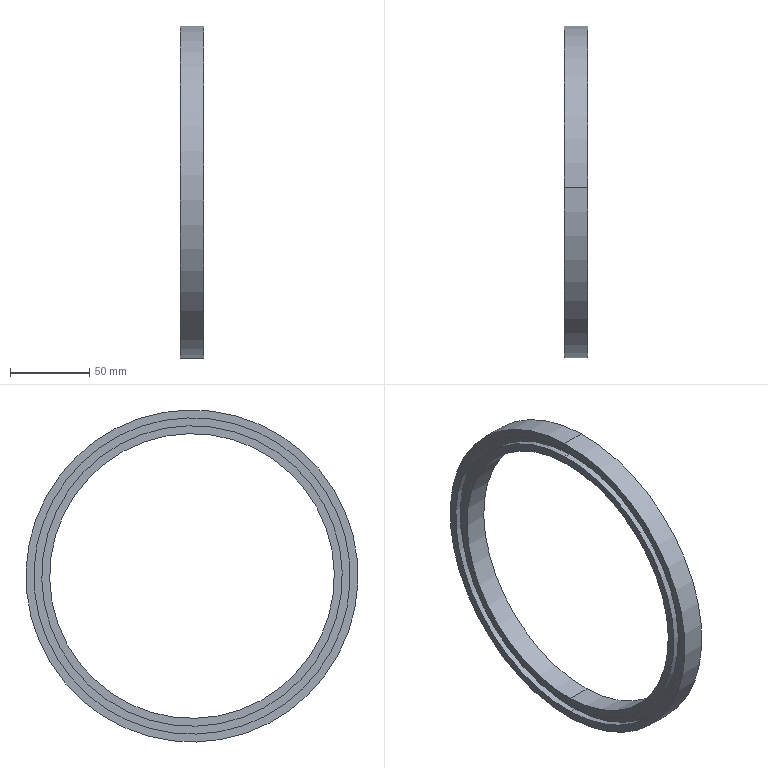Part | NX | features BREP 1 | 1 solid | 18 faces | box 15 x 210 x 210 mm | volume 113333 mm3 | cylinder 12 | plane 6 | commonest cylinder face diameters 190 x4 200 x4 180 x2 210 x2
STEP:
#1=CARTESIAN_POINT('',(-426.355,2.532,94.966));
#2=VERTEX_POINT('',#1);
#3=CARTESIAN_POINT('',(-426.355,-2.532,-94.966));
#4=VERTEX_POINT('',#3);
#5=CARTESIAN_POINT('',(-426.355,0.,0.));
#6=DIRECTION('',(1.,0.,0.));
#7=DIRECTION('',(0.,0.02665,0.9996));
#8=AXIS2_PLACEMENT_3D('',#5,#6,#7);
#9=CIRCLE('',#8,95.);
#10=EDGE_CURVE('',#2,#4,#9,.T.);
#11=ORIENTED_EDGE('',*,*,#10,.T.);
#12=CARTESIAN_POINT('',(-422.355,-2.532,-94.966));
#13=VERTEX_POINT('',#12);
#14=CARTESIAN_POINT('',(-429.855,-2.532,-94.966));
#15=DIRECTION('',(-1.,0.,0.));
#16=VECTOR('',#15,1000.);
#17=LINE('',#14,#16);
#18=EDGE_CURVE('',#4,#13,#17,.F.);
#19=ORIENTED_EDGE('',*,*,#18,.T.);
#20=CARTESIAN_POINT('',(-422.355,2.532,94.966));
#21=VERTEX_POINT('',#20);
#22=CARTESIAN_POINT('',(-422.355,0.,0.));
#23=DIRECTION('',(1.,0.,0.));
#24=DIRECTION('',(0.,0.02665,0.9996));
#25=AXIS2_PLACEMENT_3D('',#22,#23,#24);
#26=CIRCLE('',#25,95.);
#27=EDGE_CURVE('',#21,#13,#26,.T.);
#28=ORIENTED_EDGE('',*,*,#27,.F.);
#29=CARTESIAN_POINT('',(-429.855,2.532,94.966));
#30=DIRECTION('',(-1.,0.,0.));
#31=VECTOR('',#30,1000.);
#32=LINE('',#29,#31);
#33=EDGE_CURVE('',#2,#21,#32,.F.);
#34=ORIENTED_EDGE('',*,*,#33,.F.);
#35=EDGE_LOOP('',(#11,#19,#28,#34));
#36=FACE_BOUND('',#35,.T.);
#37=CARTESIAN_POINT('',(-429.855,0.,0.));
#38=DIRECTION('',(1.,0.,0.));
#39=DIRECTION('',(0.,0.02665,0.9996));
#40=AXIS2_PLACEMENT_3D('',#37,#38,#39);
#41=CYLINDRICAL_SURFACE('',#40,95.);
#42=ADVANCED_FACE('',(#36),#41,.T.);
#43=CARTESIAN_POINT('',(-426.355,-2.665,-99.964));
#44=VERTEX_POINT('',#43);
#45=CARTESIAN_POINT('',(-426.355,2.665,99.964));
#46=VERTEX_POINT('',#45);
#47=CARTESIAN_POINT('',(-426.355,0.,0.));
#48=DIRECTION('',(1.,0.,0.));
#49=DIRECTION('',(0.,0.02665,0.9996));
#50=AXIS2_PLACEMENT_3D('',#47,#48,#49);
#51=CIRCLE('',#50,100.);
#52=EDGE_CURVE('',#44,#46,#51,.T.);
#53=ORIENTED_EDGE('',*,*,#52,.F.);
#54=CARTESIAN_POINT('',(-422.355,-2.665,-99.964));
#55=VERTEX_POINT('',#54);
#56=CARTESIAN_POINT('',(-429.855,-2.665,-99.964));
#57=DIRECTION('',(-1.,0.,0.));
#58=VECTOR('',#57,1000.);
#59=LINE('',#56,#58);
#60=EDGE_CURVE('',#44,#55,#59,.F.);
#61=ORIENTED_EDGE('',*,*,#60,.T.);
#62=CARTESIAN_POINT('',(-422.355,2.665,99.964));
#63=VERTEX_POINT('',#62);
#64=CARTESIAN_POINT('',(-422.355,0.,0.));
#65=DIRECTION('',(1.,0.,0.));
#66=DIRECTION('',(0.,0.02665,0.9996));
#67=AXIS2_PLACEMENT_3D('',#64,#65,#66);
#68=CIRCLE('',#67,100.);
#69=EDGE_CURVE('',#55,#63,#68,.T.);
#70=ORIENTED_EDGE('',*,*,#69,.T.);
#71=CARTESIAN_POINT('',(-429.855,2.665,99.964));
#72=DIRECTION('',(-1.,0.,0.));
#73=VECTOR('',#72,1000.);
#74=LINE('',#71,#73);
#75=EDGE_CURVE('',#46,#63,#74,.F.);
#76=ORIENTED_EDGE('',*,*,#75,.F.);
#77=EDGE_LOOP('',(#53,#61,#70,#76));
#78=FACE_BOUND('',#77,.T.);
#79=CARTESIAN_POINT('',(-429.855,0.,0.));
#80=DIRECTION('',(1.,0.,0.));
#81=DIRECTION('',(0.,0.02665,0.9996));
#82=AXIS2_PLACEMENT_3D('',#79,#80,#81);
#83=CYLINDRICAL_SURFACE('',#82,100.);
#84=ADVANCED_FACE('',(#78),#83,.F.);
#85=CARTESIAN_POINT('',(-437.355,2.798,104.963));
#86=VERTEX_POINT('',#85);
#87=CARTESIAN_POINT('',(-437.355,-2.798,-104.963));
#88=VERTEX_POINT('',#87);
#89=CARTESIAN_POINT('',(-437.355,0.,0.));
#90=DIRECTION('',(1.,0.,0.));
#91=DIRECTION('',(0.,0.02665,0.9996));
#92=AXIS2_PLACEMENT_3D('',#89,#90,#91);
#93=CIRCLE('',#92,105.);
#94=EDGE_CURVE('',#86,#88,#93,.T.);
#95=ORIENTED_EDGE('',*,*,#94,.T.);
#96=CARTESIAN_POINT('',(-422.355,-2.798,-104.963));
#97=VERTEX_POINT('',#96);
#98=CARTESIAN_POINT('',(-429.855,-2.798,-104.963));
#99=DIRECTION('',(-1.,0.,0.));
#100=VECTOR('',#99,1000.);
#101=LINE('',#98,#100);
#102=EDGE_CURVE('',#88,#97,#101,.F.);
#103=ORIENTED_EDGE('',*,*,#102,.T.);
#104=CARTESIAN_POINT('',(-422.355,2.798,104.963));
#105=VERTEX_POINT('',#104);
#106=CARTESIAN_POINT('',(-422.355,0.,0.));
#107=DIRECTION('',(1.,0.,0.));
#108=DIRECTION('',(0.,0.02665,0.9996));
#109=AXIS2_PLACEMENT_3D('',#106,#107,#108);
#110=CIRCLE('',#109,105.);
#111=EDGE_CURVE('',#105,#97,#110,.T.);
#112=ORIENTED_EDGE('',*,*,#111,.F.);
#113=CARTESIAN_POINT('',(-429.855,2.798,104.963));
#114=DIRECTION('',(-1.,0.,0.));
#115=VECTOR('',#114,1000.);
#116=LINE('',#113,#115);
#117=EDGE_CURVE('',#86,#105,#116,.F.);
#118=ORIENTED_EDGE('',*,*,#117,.F.);
#119=EDGE_LOOP('',(#95,#103,#112,#118));
#120=FACE_BOUND('',#119,.T.);
#121=CARTESIAN_POINT('',(-429.855,0.,0.));
#122=DIRECTION('',(1.,0.,0.));
#123=DIRECTION('',(0.,0.02665,0.9996));
#124=AXIS2_PLACEMENT_3D('',#121,#122,#123);
#125=CYLINDRICAL_SURFACE('',#124,105.);
#126=ADVANCED_FACE('',(#120),#125,.T.);
#127=CARTESIAN_POINT('',(-437.355,-2.665,-99.964));
#128=VERTEX_POINT('',#127);
#129=CARTESIAN_POINT('',(-437.355,2.665,99.964));
#130=VERTEX_POINT('',#129);
#131=CARTESIAN_POINT('',(-437.355,0.,0.));
#132=DIRECTION('',(1.,0.,0.));
#133=DIRECTION('',(0.,0.02665,0.9996));
#134=AXIS2_PLACEMENT_3D('',#131,#132,#133);
#135=CIRCLE('',#134,100.);
#136=EDGE_CURVE('',#128,#130,#135,.T.);
#137=ORIENTED_EDGE('',*,*,#136,.F.);
#138=CARTESIAN_POINT('',(-433.355,-2.665,-99.964));
#139=VERTEX_POINT('',#138);
#140=CARTESIAN_POINT('',(-429.855,-2.665,-99.964));
#141=DIRECTION('',(-1.,0.,0.));
#142=VECTOR('',#141,1000.);
#143=LINE('',#140,#142);
#144=EDGE_CURVE('',#128,#139,#143,.F.);
#145=ORIENTED_EDGE('',*,*,#144,.T.);
#146=CARTESIAN_POINT('',(-433.355,2.665,99.964));
#147=VERTEX_POINT('',#146);
#148=CARTESIAN_POINT('',(-433.355,0.,0.));
#149=DIRECTION('',(1.,0.,0.));
#150=DIRECTION('',(0.,0.02665,0.9996));
#151=AXIS2_PLACEMENT_3D('',#148,#149,#150);
#152=CIRCLE('',#151,100.);
#153=EDGE_CURVE('',#139,#147,#152,.T.);
#154=ORIENTED_EDGE('',*,*,#153,.T.);
#155=CARTESIAN_POINT('',(-429.855,2.665,99.964));
#156=DIRECTION('',(-1.,0.,0.));
#157=VECTOR('',#156,1000.);
#158=LINE('',#155,#157);
#159=EDGE_CURVE('',#130,#147,#158,.F.);
#160=ORIENTED_EDGE('',*,*,#159,.F.);
#161=EDGE_LOOP('',(#137,#145,#154,#160));
#162=FACE_BOUND('',#161,.T.);
#163=CARTESIAN_POINT('',(-429.855,0.,0.));
#164=DIRECTION('',(1.,0.,0.));
#165=DIRECTION('',(0.,0.02665,0.9996));
#166=AXIS2_PLACEMENT_3D('',#163,#164,#165);
#167=CYLINDRICAL_SURFACE('',#166,100.);
#168=ADVANCED_FACE('',(#162),#167,.F.);
#169=CARTESIAN_POINT('',(-437.355,2.532,94.966));
#170=VERTEX_POINT('',#169);
#171=CARTESIAN_POINT('',(-437.355,-2.532,-94.966));
#172=VERTEX_POINT('',#171);
#173=CARTESIAN_POINT('',(-437.355,0.,0.));
#174=DIRECTION('',(1.,0.,0.));
#175=DIRECTION('',(0.,0.02665,0.9996));
#176=AXIS2_PLACEMENT_3D('',#173,#174,#175);
#177=CIRCLE('',#176,95.);
#178=EDGE_CURVE('',#170,#172,#177,.T.);
#179=ORIENTED_EDGE('',*,*,#178,.T.);
#180=CARTESIAN_POINT('',(-433.355,-2.532,-94.966));
#181=VERTEX_POINT('',#180);
#182=CARTESIAN_POINT('',(-429.855,-2.532,-94.966));
#183=DIRECTION('',(-1.,0.,0.));
#184=VECTOR('',#183,1000.);
#185=LINE('',#182,#184);
#186=EDGE_CURVE('',#172,#181,#185,.F.);
#187=ORIENTED_EDGE('',*,*,#186,.T.);
#188=CARTESIAN_POINT('',(-433.355,2.532,94.966));
#189=VERTEX_POINT('',#188);
#190=CARTESIAN_POINT('',(-433.355,0.,0.));
#191=DIRECTION('',(1.,0.,0.));
#192=DIRECTION('',(0.,0.02665,0.9996));
#193=AXIS2_PLACEMENT_3D('',#190,#191,#192);
#194=CIRCLE('',#193,95.);
#195=EDGE_CURVE('',#189,#181,#194,.T.);
#196=ORIENTED_EDGE('',*,*,#195,.F.);
#197=CARTESIAN_POINT('',(-429.855,2.532,94.966));
#198=DIRECTION('',(-1.,0.,0.));
#199=VECTOR('',#198,1000.);
#200=LINE('',#197,#199);
#201=EDGE_CURVE('',#170,#189,#200,.F.);
#202=ORIENTED_EDGE('',*,*,#201,.F.);
#203=EDGE_LOOP('',(#179,#187,#196,#202));
#204=FACE_BOUND('',#203,.T.);
#205=CARTESIAN_POINT('',(-429.855,0.,0.));
#206=DIRECTION('',(1.,0.,0.));
#207=DIRECTION('',(0.,0.02665,0.9996));
#208=AXIS2_PLACEMENT_3D('',#205,#206,#207);
#209=CYLINDRICAL_SURFACE('',#208,95.);
#210=ADVANCED_FACE('',(#204),#209,.T.);
#211=CARTESIAN_POINT('',(-437.355,-2.399,-89.968));
#212=VERTEX_POINT('',#211);
#213=CARTESIAN_POINT('',(-437.355,2.399,89.968));
#214=VERTEX_POINT('',#213);
#215=CARTESIAN_POINT('',(-437.355,0.,0.));
#216=DIRECTION('',(1.,0.,0.));
#217=DIRECTION('',(0.,0.02665,0.9996));
#218=AXIS2_PLACEMENT_3D('',#215,#216,#217);
#219=CIRCLE('',#218,90.);
#220=EDGE_CURVE('',#212,#214,#219,.T.);
#221=ORIENTED_EDGE('',*,*,#220,.F.);
#222=CARTESIAN_POINT('',(-422.355,-2.399,-89.968));
#223=VERTEX_POINT('',#222);
#224=CARTESIAN_POINT('',(-429.855,-2.399,-89.968));
#225=DIRECTION('',(-1.,0.,0.));
#226=VECTOR('',#225,1000.);
#227=LINE('',#224,#226);
#228=EDGE_CURVE('',#212,#223,#227,.F.);
#229=ORIENTED_EDGE('',*,*,#228,.T.);
#230=CARTESIAN_POINT('',(-422.355,2.399,89.968));
#231=VERTEX_POINT('',#230);
#232=CARTESIAN_POINT('',(-422.355,0.,0.));
#233=DIRECTION('',(1.,0.,0.));
#234=DIRECTION('',(0.,0.02665,0.9996));
#235=AXIS2_PLACEMENT_3D('',#232,#233,#234);
#236=CIRCLE('',#235,90.);
#237=EDGE_CURVE('',#223,#231,#236,.T.);
#238=ORIENTED_EDGE('',*,*,#237,.T.);
#239=CARTESIAN_POINT('',(-429.855,2.399,89.968));
#240=DIRECTION('',(-1.,0.,0.));
#241=VECTOR('',#240,1000.);
#242=LINE('',#239,#241);
#243=EDGE_CURVE('',#214,#231,#242,.F.);
#244=ORIENTED_EDGE('',*,*,#243,.F.);
#245=EDGE_LOOP('',(#221,#229,#238,#244));
#246=FACE_BOUND('',#245,.T.);
#247=CARTESIAN_POINT('',(-429.855,0.,0.));
#248=DIRECTION('',(1.,0.,0.));
#249=DIRECTION('',(0.,0.02665,0.9996));
#250=AXIS2_PLACEMENT_3D('',#247,#248,#249);
#251=CYLINDRICAL_SURFACE('',#250,90.);
#252=ADVANCED_FACE('',(#246),#251,.F.);
#253=ORIENTED_EDGE('',*,*,#228,.F.);
#254=CARTESIAN_POINT('',(-437.355,0.,0.));
#255=DIRECTION('',(1.,0.,0.));
#256=DIRECTION('',(0.,0.02665,0.9996));
#257=AXIS2_PLACEMENT_3D('',#254,#255,#256);
#258=CIRCLE('',#257,90.);
#259=EDGE_CURVE('',#214,#212,#258,.T.);
#260=ORIENTED_EDGE('',*,*,#259,.F.);
#261=ORIENTED_EDGE('',*,*,#243,.T.);
#262=CARTESIAN_POINT('',(-422.355,0.,0.));
#263=DIRECTION('',(1.,0.,0.));
#264=DIRECTION('',(0.,0.02665,0.9996));
#265=AXIS2_PLACEMENT_3D('',#262,#263,#264);
#266=CIRCLE('',#265,90.);
#267=EDGE_CURVE('',#231,#223,#266,.T.);
#268=ORIENTED_EDGE('',*,*,#267,.T.);
#269=EDGE_LOOP('',(#253,#260,#261,#268));
#270=FACE_BOUND('',#269,.T.);
#271=CARTESIAN_POINT('',(-429.855,0.,0.));
#272=DIRECTION('',(1.,0.,0.));
#273=DIRECTION('',(0.,0.02665,0.9996));
#274=AXIS2_PLACEMENT_3D('',#271,#272,#273);
#275=CYLINDRICAL_SURFACE('',#274,90.);
#276=ADVANCED_FACE('',(#270),#275,.F.);
#277=ORIENTED_EDGE('',*,*,#178,.F.);
#278=CARTESIAN_POINT('',(-437.355,0.,0.));
#279=DIRECTION('',(1.,0.,0.));
#280=DIRECTION('',(0.,0.02665,0.9996));
#281=AXIS2_PLACEMENT_3D('',#278,#279,#280);
#282=CIRCLE('',#281,95.);
#283=EDGE_CURVE('',#172,#170,#282,.T.);
#284=ORIENTED_EDGE('',*,*,#283,.F.);
#285=EDGE_LOOP('',(#277,#284));
#286=FACE_BOUND('',#285,.T.);
#287=ORIENTED_EDGE('',*,*,#259,.T.);
#288=ORIENTED_EDGE('',*,*,#220,.T.);
#289=EDGE_LOOP('',(#287,#288));
#290=FACE_BOUND('',#289,.T.);
#291=CARTESIAN_POINT('',(-437.355,-89.968,2.399));
#292=DIRECTION('',(1.,0.,0.));
#293=DIRECTION('',(0.,0.02665,0.9996));
#294=AXIS2_PLACEMENT_3D('',#291,#292,#293);
#295=PLANE('',#294);
#296=ADVANCED_FACE('',(#286,#290),#295,.F.);
#297=ORIENTED_EDGE('',*,*,#186,.F.);
#298=ORIENTED_EDGE('',*,*,#283,.T.);
#299=ORIENTED_EDGE('',*,*,#201,.T.);
#300=CARTESIAN_POINT('',(-433.355,0.,0.));
#301=DIRECTION('',(1.,0.,0.));
#302=DIRECTION('',(0.,0.02665,0.9996));
#303=AXIS2_PLACEMENT_3D('',#300,#301,#302);
#304=CIRCLE('',#303,95.);
#305=EDGE_CURVE('',#181,#189,#304,.T.);
#306=ORIENTED_EDGE('',*,*,#305,.F.);
#307=EDGE_LOOP('',(#297,#298,#299,#306));
#308=FACE_BOUND('',#307,.T.);
#309=CARTESIAN_POINT('',(-429.855,0.,0.));
#310=DIRECTION('',(1.,0.,0.));
#311=DIRECTION('',(0.,0.02665,0.9996));
#312=AXIS2_PLACEMENT_3D('',#309,#310,#311);
#313=CYLINDRICAL_SURFACE('',#312,95.);
#314=ADVANCED_FACE('',(#308),#313,.T.);
#315=CARTESIAN_POINT('',(-433.355,0.,0.));
#316=DIRECTION('',(1.,0.,0.));
#317=DIRECTION('',(0.,0.02665,0.9996));
#318=AXIS2_PLACEMENT_3D('',#315,#316,#317);
#319=CIRCLE('',#318,100.);
#320=EDGE_CURVE('',#147,#139,#319,.T.);
#321=ORIENTED_EDGE('',*,*,#320,.F.);
#322=ORIENTED_EDGE('',*,*,#153,.F.);
#323=EDGE_LOOP('',(#321,#322));
#324=FACE_BOUND('',#323,.T.);
#325=ORIENTED_EDGE('',*,*,#195,.T.);
#326=ORIENTED_EDGE('',*,*,#305,.T.);
#327=EDGE_LOOP('',(#325,#326));
#328=FACE_BOUND('',#327,.T.);
#329=CARTESIAN_POINT('',(-433.355,-94.966,2.532));
#330=DIRECTION('',(1.,0.,0.));
#331=DIRECTION('',(0.,0.02665,0.9996));
#332=AXIS2_PLACEMENT_3D('',#329,#330,#331);
#333=PLANE('',#332);
#334=ADVANCED_FACE('',(#324,#328),#333,.F.);
#335=ORIENTED_EDGE('',*,*,#144,.F.);
#336=CARTESIAN_POINT('',(-437.355,0.,0.));
#337=DIRECTION('',(1.,0.,0.));
#338=DIRECTION('',(0.,0.02665,0.9996));
#339=AXIS2_PLACEMENT_3D('',#336,#337,#338);
#340=CIRCLE('',#339,100.);
#341=EDGE_CURVE('',#130,#128,#340,.T.);
#342=ORIENTED_EDGE('',*,*,#341,.F.);
#343=ORIENTED_EDGE('',*,*,#159,.T.);
#344=ORIENTED_EDGE('',*,*,#320,.T.);
#345=EDGE_LOOP('',(#335,#342,#343,#344));
#346=FACE_BOUND('',#345,.T.);
#347=CARTESIAN_POINT('',(-429.855,0.,0.));
#348=DIRECTION('',(1.,0.,0.));
#349=DIRECTION('',(0.,0.02665,0.9996));
#350=AXIS2_PLACEMENT_3D('',#347,#348,#349);
#351=CYLINDRICAL_SURFACE('',#350,100.);
#352=ADVANCED_FACE('',(#346),#351,.F.);
#353=ORIENTED_EDGE('',*,*,#94,.F.);
#354=CARTESIAN_POINT('',(-437.355,0.,0.));
#355=DIRECTION('',(1.,0.,0.));
#356=DIRECTION('',(0.,0.02665,0.9996));
#357=AXIS2_PLACEMENT_3D('',#354,#355,#356);
#358=CIRCLE('',#357,105.);
#359=EDGE_CURVE('',#88,#86,#358,.T.);
#360=ORIENTED_EDGE('',*,*,#359,.F.);
#361=EDGE_LOOP('',(#353,#360));
#362=FACE_BOUND('',#361,.T.);
#363=ORIENTED_EDGE('',*,*,#341,.T.);
#364=ORIENTED_EDGE('',*,*,#136,.T.);
#365=EDGE_LOOP('',(#363,#364));
#366=FACE_BOUND('',#365,.T.);
#367=CARTESIAN_POINT('',(-437.355,-99.964,2.665));
#368=DIRECTION('',(1.,0.,0.));
#369=DIRECTION('',(0.,0.02665,0.9996));
#370=AXIS2_PLACEMENT_3D('',#367,#368,#369);
#371=PLANE('',#370);
#372=ADVANCED_FACE('',(#362,#366),#371,.F.);
#373=ORIENTED_EDGE('',*,*,#102,.F.);
#374=ORIENTED_EDGE('',*,*,#359,.T.);
#375=ORIENTED_EDGE('',*,*,#117,.T.);
#376=CARTESIAN_POINT('',(-422.355,0.,0.));
#377=DIRECTION('',(1.,0.,0.));
#378=DIRECTION('',(0.,0.02665,0.9996));
#379=AXIS2_PLACEMENT_3D('',#376,#377,#378);
#380=CIRCLE('',#379,105.);
#381=EDGE_CURVE('',#97,#105,#380,.T.);
#382=ORIENTED_EDGE('',*,*,#381,.F.);
#383=EDGE_LOOP('',(#373,#374,#375,#382));
#384=FACE_BOUND('',#383,.T.);
#385=CARTESIAN_POINT('',(-429.855,0.,0.));
#386=DIRECTION('',(1.,0.,0.));
#387=DIRECTION('',(0.,0.02665,0.9996));
#388=AXIS2_PLACEMENT_3D('',#385,#386,#387);
#389=CYLINDRICAL_SURFACE('',#388,105.);
#390=ADVANCED_FACE('',(#384),#389,.T.);
#391=CARTESIAN_POINT('',(-422.355,0.,0.));
#392=DIRECTION('',(1.,0.,0.));
#393=DIRECTION('',(0.,0.02665,0.9996));
#394=AXIS2_PLACEMENT_3D('',#391,#392,#393);
#395=CIRCLE('',#394,100.);
#396=EDGE_CURVE('',#63,#55,#395,.T.);
#397=ORIENTED_EDGE('',*,*,#396,.F.);
#398=ORIENTED_EDGE('',*,*,#69,.F.);
#399=EDGE_LOOP('',(#397,#398));
#400=FACE_BOUND('',#399,.T.);
#401=ORIENTED_EDGE('',*,*,#111,.T.);
#402=ORIENTED_EDGE('',*,*,#381,.T.);
#403=EDGE_LOOP('',(#401,#402));
#404=FACE_BOUND('',#403,.T.);
#405=CARTESIAN_POINT('',(-422.355,-104.963,2.798));
#406=DIRECTION('',(-1.,0.,0.));
#407=DIRECTION('',(0.,-0.02665,-0.9996));
#408=AXIS2_PLACEMENT_3D('',#405,#406,#407);
#409=PLANE('',#408);
#410=ADVANCED_FACE('',(#400,#404),#409,.F.);
#411=ORIENTED_EDGE('',*,*,#60,.F.);
#412=CARTESIAN_POINT('',(-426.355,0.,0.));
#413=DIRECTION('',(1.,0.,0.));
#414=DIRECTION('',(0.,0.02665,0.9996));
#415=AXIS2_PLACEMENT_3D('',#412,#413,#414);
#416=CIRCLE('',#415,100.);
#417=EDGE_CURVE('',#46,#44,#416,.T.);
#418=ORIENTED_EDGE('',*,*,#417,.F.);
#419=ORIENTED_EDGE('',*,*,#75,.T.);
#420=ORIENTED_EDGE('',*,*,#396,.T.);
#421=EDGE_LOOP('',(#411,#418,#419,#420));
#422=FACE_BOUND('',#421,.T.);
#423=CARTESIAN_POINT('',(-429.855,0.,0.));
#424=DIRECTION('',(1.,0.,0.));
#425=DIRECTION('',(0.,0.02665,0.9996));
#426=AXIS2_PLACEMENT_3D('',#423,#424,#425);
#427=CYLINDRICAL_SURFACE('',#426,100.);
#428=ADVANCED_FACE('',(#422),#427,.F.);
#429=ORIENTED_EDGE('',*,*,#10,.F.);
#430=CARTESIAN_POINT('',(-426.355,0.,0.));
#431=DIRECTION('',(1.,0.,0.));
#432=DIRECTION('',(0.,0.02665,0.9996));
#433=AXIS2_PLACEMENT_3D('',#430,#431,#432);
#434=CIRCLE('',#433,95.);
#435=EDGE_CURVE('',#4,#2,#434,.T.);
#436=ORIENTED_EDGE('',*,*,#435,.F.);
#437=EDGE_LOOP('',(#429,#436));
#438=FACE_BOUND('',#437,.T.);
#439=ORIENTED_EDGE('',*,*,#417,.T.);
#440=ORIENTED_EDGE('',*,*,#52,.T.);
#441=EDGE_LOOP('',(#439,#440));
#442=FACE_BOUND('',#441,.T.);
#443=CARTESIAN_POINT('',(-426.355,-99.964,2.665));
#444=DIRECTION('',(-1.,0.,0.));
#445=DIRECTION('',(0.,-0.02665,-0.9996));
#446=AXIS2_PLACEMENT_3D('',#443,#444,#445);
#447=PLANE('',#446);
#448=ADVANCED_FACE('',(#438,#442),#447,.F.);
#449=ORIENTED_EDGE('',*,*,#18,.F.);
#450=ORIENTED_EDGE('',*,*,#435,.T.);
#451=ORIENTED_EDGE('',*,*,#33,.T.);
#452=CARTESIAN_POINT('',(-422.355,0.,0.));
#453=DIRECTION('',(1.,0.,0.));
#454=DIRECTION('',(0.,0.02665,0.9996));
#455=AXIS2_PLACEMENT_3D('',#452,#453,#454);
#456=CIRCLE('',#455,95.);
#457=EDGE_CURVE('',#13,#21,#456,.T.);
#458=ORIENTED_EDGE('',*,*,#457,.F.);
#459=EDGE_LOOP('',(#449,#450,#451,#458));
#460=FACE_BOUND('',#459,.T.);
#461=CARTESIAN_POINT('',(-429.855,0.,0.));
#462=DIRECTION('',(1.,0.,0.));
#463=DIRECTION('',(0.,0.02665,0.9996));
#464=AXIS2_PLACEMENT_3D('',#461,#462,#463);
#465=CYLINDRICAL_SURFACE('',#464,95.);
#466=ADVANCED_FACE('',(#460),#465,.T.);
#467=ORIENTED_EDGE('',*,*,#267,.F.);
#468=ORIENTED_EDGE('',*,*,#237,.F.);
#469=EDGE_LOOP('',(#467,#468));
#470=FACE_BOUND('',#469,.T.);
#471=ORIENTED_EDGE('',*,*,#27,.T.);
#472=ORIENTED_EDGE('',*,*,#457,.T.);
#473=EDGE_LOOP('',(#471,#472));
#474=FACE_BOUND('',#473,.T.);
#475=CARTESIAN_POINT('',(-422.355,-94.966,2.532));
#476=DIRECTION('',(-1.,0.,0.));
#477=DIRECTION('',(0.,-0.02665,-0.9996));
#478=AXIS2_PLACEMENT_3D('',#475,#476,#477);
#479=PLANE('',#478);
#480=ADVANCED_FACE('',(#470,#474),#479,.F.);
#481=CLOSED_SHELL('',(#42,#84,#126,#168,#210,#252,#276,#296,#314,#334,#352,#372,#390,#410,#428,#448,#466,#480));
#482=MANIFOLD_SOLID_BREP('',#481);
#483=(LENGTH_UNIT()NAMED_UNIT(*)SI_UNIT(.MILLI.,.METRE.));
#484=UNCERTAINTY_MEASURE_WITH_UNIT(LENGTH_MEASURE(0.00001),#483,'','');
#485=(NAMED_UNIT(*)PLANE_ANGLE_UNIT()SI_UNIT($,.RADIAN.));
#486=(NAMED_UNIT(*)SI_UNIT($,.STERADIAN.)SOLID_ANGLE_UNIT());
#487=(GEOMETRIC_REPRESENTATION_CONTEXT(3)GLOBAL_UNCERTAINTY_ASSIGNED_CONTEXT((#484))GLOBAL_UNIT_ASSIGNED_CONTEXT((#483,#485,#486))REPRESENTATION_CONTEXT('',''));
#488=ADVANCED_BREP_SHAPE_REPRESENTATION('',(#482),#487);